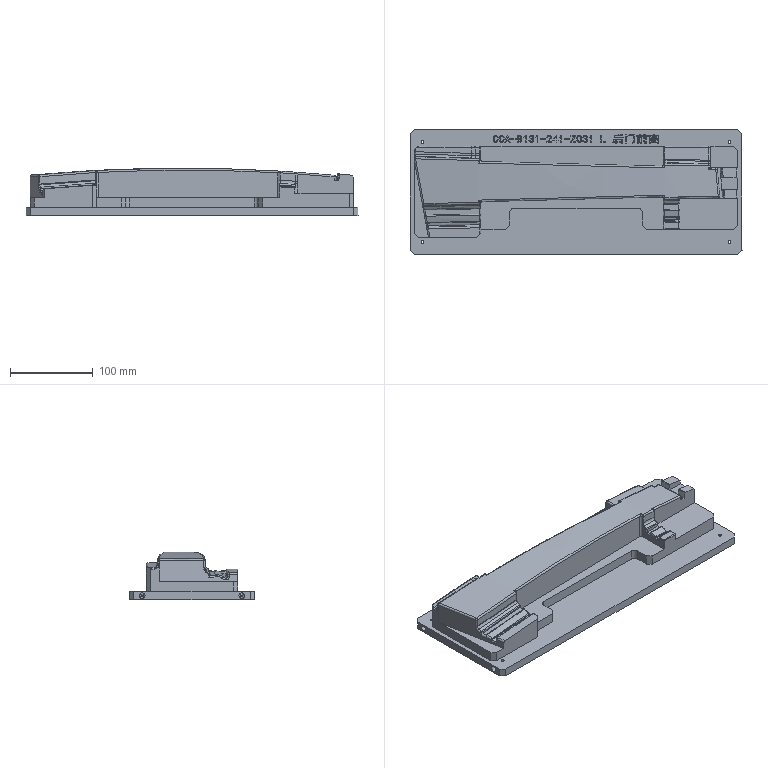NC program | NX | posted with a generic post | part box 400 x 150 x 57.494 mm
Lines 7336 to 8369 of 16235:
(B2 , TOOL : D6)
N14670 M6
N14672 G54
N14674 G17 G0 G90 X-117.012 Y45.277 S3500 M3
N14676 G43 Z69.953 H0
N14678 Z54.94
N14680 G94 G1 Z54.64 F2000.
N14682 X-115.309 Y43.211
N14684 X-113.402 Y40.898 Z54.536
N14686 G2 X-112.655 Y39.453 R3.866
N14688 X-109.882 Y39.507 R578.074
N14690 G1 X-106.884 Y39.558 Z54.64
N14692 X-106.919 Y42.55
N14694 Z54.94
N14696 G0 Z62.753
N14698 X-116.766 Y45.803
N14700 Z54.445
N14702 G1 Z54.145
N14704 X-114.899 Y43.597
N14706 X-112.963 Y41.308 Z54.041
N14708 G2 X-112.167 Y39.876 R4.223
N14710 X-109.559 Y39.87 R984.3
N14712 G1 X-106.561 Y39.859 Z54.145
N14714 X-106.541 Y42.854
N14716 Z54.445
N14718 G0 Z54.836
N14720 X-116.488 Y46.083
N14722 Z53.951
N14724 G1 Z53.651
N14726 X-114.599 Y43.8
N14728 X-112.687 Y41.491 Z53.546
N14730 G2 X-111.905 Y40.082 R4.383
N14732 X-109.285 Y40.044 R1249.651
N14734 G1 X-106.287 Y39.998 Z53.651
N14736 X-106.234 Y42.994
N14738 Z53.951
N14740 G0 Z54.341
N14742 X-116.36 Y46.216
N14744 Z53.456
N14746 G1 Z53.156
N14748 X-114.458 Y43.892
N14750 X-112.56 Y41.572 Z53.051
N14752 G2 X-111.787 Y40.176 R4.458
N14754 G1 X-109.211 Y40.108
N14756 X-106.213 Y40.03 Z53.156
N14758 X-106.135 Y43.029
N14760 Z53.456
N14762 G0 Z53.846
N14764 X-116.319 Y46.25
N14766 Z52.961
N14768 G1 Z52.661
N14770 X-114.409 Y43.907
N14772 X-112.514 Y41.583 Z52.556
N14774 G2 X-111.738 Y40.18 R4.504
N14776 G1 X-109.189 Y40.113
N14778 X-106.192 Y40.035 Z52.661
N14780 X-106.114 Y43.034
N14782 Z52.961
N14784 G0 Z53.351
N14786 X-116.324 Y46.252
N14788 Z52.466
N14790 G1 Z52.166
N14792 X-114.411 Y43.908
N14794 X-112.515 Y41.585 Z52.062
N14796 G2 X-111.738 Y40.18 R4.503
N14798 G1 X-109.188 Y40.113
N14800 X-106.191 Y40.035 Z52.166
N14802 X-106.113 Y43.034
N14804 Z52.466
N14806 G0 Z52.856
N14808 X-116.328 Y46.252
N14810 Z51.971
N14812 G1 Z51.671
N14814 X-114.413 Y43.909
N14816 X-112.517 Y41.587 Z51.567
N14818 G2 X-111.741 Y40.187 R4.502
N14820 G1 X-111.529 Y40.175
N14822 X-109.188 Y40.113
N14824 X-106.191 Y40.035 Z51.671
N14826 X-106.112 Y43.034
N14828 Z51.971
N14830 G0 Z52.362
N14832 X-116.331 Y46.252
N14834 Z51.477
N14836 G1 Z51.177
N14838 X-114.416 Y43.91
N14840 X-112.518 Y41.589 Z51.072
N14842 G2 X-111.741 Y40.187 R4.501
N14844 G1 X-111.529 Y40.175
N14846 X-109.187 Y40.113
N14848 X-106.19 Y40.035 Z51.177
N14850 X-106.111 Y43.034
N14852 Z51.477
N14854 G0 Z51.867
N14856 X-116.334 Y46.253
N14858 Z50.982
N14860 G1 Z50.682
N14862 X-114.418 Y43.911
N14864 X-112.519 Y41.591 Z50.577
N14866 G2 X-111.741 Y40.187 R4.5
N14868 G1 X-111.529 Y40.175
N14870 X-109.186 Y40.113
N14872 X-106.189 Y40.035 Z50.682
N14874 X-106.11 Y43.034
N14876 Z50.982
N14878 G0 Z51.372
N14880 X-116.332 Y46.251
N14882 Z50.487
N14884 G1 Z50.187
N14886 X-114.418 Y43.911
N14888 X-112.519 Y41.591 Z50.082
N14890 G2 X-111.741 Y40.187 R4.498
N14892 G1 X-111.681 Y40.177
N14894 X-111.529 Y40.172
N14896 Y40.175
N14898 X-109.186 Y40.113
N14900 X-106.189 Y40.035 Z50.187
N14902 X-106.11 Y43.034
N14904 Z50.487
N14906 G0 Z50.877
N14908 X-116.333 Y46.253
N14910 Z49.992
N14912 G1 Z49.692
N14914 X-114.418 Y43.912
N14916 X-112.519 Y41.591 Z49.587
N14918 G2 X-111.74 Y40.187 R4.497
N14920 G1 X-111.681 Y40.177
N14922 X-111.529 Y40.175
N14924 X-109.186 Y40.113
N14926 X-106.188 Y40.035 Z49.692
N14928 X-106.11 Y43.034
N14930 Z49.992
N14932 G0 Z50.382
N14934 X-116.332 Y46.253
N14936 Z49.497
N14938 G1 Z49.197
N14940 X-114.417 Y43.912
N14942 X-112.519 Y41.592 Z49.093
N14944 G2 X-111.74 Y40.187 R4.496
N14946 G1 X-111.681 Y40.177
N14948 X-111.529 Y40.175
N14950 X-109.185 Y40.113
N14952 X-106.188 Y40.035 Z49.197
N14954 X-106.11 Y43.034
N14956 Z49.497
N14958 G0 Z49.887
N14960 X-116.333 Y46.253
N14962 Z49.003
N14964 G1 Z48.703
N14966 X-114.417 Y43.912
N14968 X-112.518 Y41.591 Z48.598
N14970 G2 X-111.747 Y40.208 R4.498
N14972 G1 X-111.737 Y40.165
N14974 X-111.696 Y40.179
N14976 X-109.185 Y40.113
N14978 X-106.188 Y40.035 Z48.703
N14980 X-106.109 Y43.034
N14982 Z49.003
N14984 G0 Z49.393
N14986 X-116.331 Y46.251
N14988 Z48.508
N14990 G1 Z48.208
N14992 X-114.417 Y43.912
N14994 X-112.518 Y41.592 Z48.103
N14996 G2 X-111.746 Y40.208 R4.497
N14998 G1 X-111.737 Y40.164
N15000 X-111.695 Y40.179
N15002 X-109.185 Y40.113
N15004 X-106.187 Y40.035 Z48.208
N15006 X-106.109 Y43.034
N15008 Z48.508
N15010 G0 Z48.898
N15012 X-116.324 Y46.251
N15014 Z48.013
N15016 G1 Z47.713
N15018 X-114.413 Y43.912
N15020 X-112.516 Y41.59 Z47.608
N15022 G2 X-111.746 Y40.208 R4.494
N15024 G1 X-111.737 Y40.164
N15026 X-111.695 Y40.179
N15028 X-109.184 Y40.113
N15030 X-106.187 Y40.035 Z47.713
N15032 X-106.109 Y43.034
N15034 Z48.013
N15036 G0 Z48.403
N15038 X-116.302 Y46.271
N15040 Z47.518
N15042 G1 Z47.218
N15044 X-114.399 Y43.923
N15046 X-112.511 Y41.595 Z47.113
N15048 G2 X-111.738 Y40.188 R4.505
N15050 G1 X-111.678 Y40.179
N15052 X-109.174 Y40.113
N15054 X-106.177 Y40.035 Z47.218
N15056 X-106.098 Y43.034
N15058 Z47.518
N15060 G0 Z47.908
N15062 X-116.122 Y46.434
N15064 Z47.023
N15066 G1 Z46.723
N15068 X-114.299 Y44.065
N15070 X-112.47 Y41.69 Z46.619
N15072 G2 X-112.002 Y40.938 R4.471
N15074 G1 X-111.717 Y40.316
N15076 X-111.748 Y40.233
N15078 X-111.678 Y40.179
N15080 X-109.013 Y40.109
N15082 X-106.015 Y40.03 Z46.723
N15084 X-105.937 Y43.029
N15086 Z47.023
N15088 G0 Z47.413
N15090 X-115.811 Y46.744
N15092 Z46.528
N15094 G1 Z46.228
N15096 X-114.099 Y44.296
N15098 X-112.38 Y41.84 Z46.124
N15100 G2 X-111.86 Y40.855 R4.471
N15102 G1 X-111.656 Y40.316
N15104 X-111.642 Y40.178
N15106 X-108.697 Y40.101
N15108 X-105.699 Y40.022 Z46.228
N15110 X-105.621 Y43.021
N15112 Z46.528
N15114 G0 Z46.919
N15116 X-115.417 Y47.282
N15118 Z46.034
N15120 G1 Z45.734
N15122 X-113.898 Y44.752
N15124 X-112.354 Y42.182 Z45.629
N15126 X-112.236 Y41.987
N15128 G2 X-111.576 Y40.176 R5.063
N15130 G1 X-108.345 Y40.092
N15132 X-105.348 Y40.013 Z45.734
N15134 X-105.27 Y43.012
N15136 Z46.034
N15138 G0 Z46.424
N15140 X-115.223 Y48.184
N15142 Z45.539
N15144 G1 Z45.239
N15146 X-113.671 Y45.306
N15148 X-112.249 Y42.667 Z45.134
N15150 G2 X-111.524 Y40.224 R6.224
N15152 G1 X-111.54 Y40.181
N15154 X-111.503 Y40.149
N15156 X-111.462 Y40.17
N15158 X-107.74 Y40.073
N15160 X-104.743 Y39.994 Z45.239
N15162 X-104.664 Y42.993
N15164 Z45.539
N15166 G0 Z45.929
N15168 X-109.191 Y48.973
N15170 Z45.044
N15172 G1 Z44.744
N15174 X-112.19 Y48.917
N15176 X-112.134 Y45.919 Z44.639
N15178 X-112.093 Y43.733
N15180 X-112.056 Y43.424
N15182 G2 X-111.5 Y40.29 R12.132
N15184 G1 Y40.175
N15186 X-106.26 Y40.038
N15188 X-103.262 Y39.959 Z44.744
N15190 X-103.184 Y42.958
N15192 Z45.044
N15194 G0 Z45.434
N15196 X-108.67 Y49.116
N15198 Z44.549
N15200 G1 Z44.249
N15202 X-111.67 Y49.102
N15204 X-111.656 Y46.104 Z44.144
N15206 X-111.644 Y43.424
N15208 X-111.515 Y41.559
N15210 X-111.5 Y41.107
N15212 Y40.175
N15214 X-105.75 Y40.024
N15216 X-102.753 Y39.946 Z44.249
N15218 X-102.674 Y42.945
N15220 Z44.549
N15222 G0 Z44.939
N15224 X-108.509 Y49.092
N15226 Z44.054
N15228 G1 Z43.754
N15230 X-111.509 Y49.088
N15232 X-111.506 Y46.09 Z43.65
N15234 X-111.502 Y42.802
N15236 X-111.5 Y42.704
N15238 Y40.175
N15240 X-105.601 Y40.02
N15242 X-102.604 Y39.942 Z43.754
N15244 X-102.525 Y42.941
N15246 Z44.054
N15248 G0 Z44.444
N15250 X-108.5 Y49.074
N15252 Z43.56
N15254 G1 Z43.26
N15256 X-111.5
N15258 Y46.076 Z43.155
N15260 Y40.175
N15262 X-105.601 Y40.02
N15264 X-102.604 Y39.942 Z43.26
N15266 X-102.525 Y42.941
N15268 Z43.56
N15270 G0 Z43.95
N15272 X-108.5 Y49.074
N15274 Z43.065
N15276 G1 Z42.765
N15278 X-111.5
N15280 Y46.076 Z42.66
N15282 Y40.175
N15284 X-105.601 Y40.02
N15286 X-102.603 Y39.942 Z42.765
N15288 X-102.525 Y42.941
N15290 Z43.065
N15292 G0 Z43.455
N15294 X-108.5 Y49.074
N15296 Z42.57
N15298 G1 Z42.27
N15300 X-111.5
N15302 Y46.076 Z42.165
N15304 Y40.175
N15306 X-105.6 Y40.02
N15308 X-102.603 Y39.942 Z42.27
N15310 X-102.525 Y42.941
N15312 Z42.57
N15314 G0 Z42.96
N15316 X-108.5 Y49.074
N15318 Z42.075
N15320 G1 Z41.775
N15322 X-111.5
N15324 Y46.076 Z41.67
N15326 Y40.175
N15328 X-105.6 Y40.02
N15330 X-102.603 Y39.942 Z41.775
N15332 X-102.524 Y42.941
N15334 Z42.075
N15336 G0 Z42.465
N15338 X-108.5 Y49.074
N15340 Z41.58
N15342 G1 Z41.28
N15344 X-111.5
N15346 Y46.076 Z41.176
N15348 Y40.175
N15350 X-105.6 Y40.02
N15352 X-102.603 Y39.942 Z41.28
N15354 X-102.524 Y42.941
N15356 Z41.58
N15358 G0 Z41.97
N15360 X-108.5 Y49.074
N15362 Z41.085
N15364 G1 Z40.785
N15366 X-111.5
N15368 Y46.076 Z40.681
N15370 Y40.175
N15372 X-105.6 Y40.02
N15374 X-102.603 Y39.942 Z40.785
N15376 X-102.524 Y42.941
N15378 Z41.085
N15380 G0 Z41.476
N15382 X-108.5 Y49.074
N15384 Z40.591
N15386 G1 Z40.291
N15388 X-111.5
N15390 Y46.076 Z40.186
N15392 Y40.175
N15394 X-105.6 Y40.02
N15396 X-102.602 Y39.942 Z40.291
N15398 X-102.524 Y42.941
N15400 Z40.591
N15402 G0 Z40.981
N15404 X-108.5 Y49.074
N15406 Z40.096
N15408 G1 Z39.796
N15410 X-111.5
N15412 Y46.076 Z39.691
N15414 Y40.175
N15416 X-105.599 Y40.02
N15418 X-102.602 Y39.942 Z39.796
N15420 X-102.524 Y42.941
N15422 Z40.096
N15424 G0 Z40.486
N15426 X-108.5 Y49.074
N15428 Z39.601
N15430 G1 Z39.301
N15432 X-111.5
N15434 Y46.076 Z39.196
N15436 Y40.175
N15438 X-105.599 Y40.02
N15440 X-102.602 Y39.942 Z39.301
N15442 X-102.524 Y42.941
N15444 Z39.601
N15446 G0 Z39.991
N15448 X-108.5 Y49.074
N15450 Z39.106
N15452 G1 Z38.806
N15454 X-111.5
N15456 Y46.076 Z38.702
N15458 Y40.175
N15460 X-105.599 Y40.02
N15462 X-102.602 Y39.942 Z38.806
N15464 X-102.523 Y42.941
N15466 Z39.106
N15468 G0 Z39.496
N15470 X-108.5 Y49.074
N15472 Z38.611
N15474 G1 Z38.311
N15476 X-111.5
N15478 Y46.076 Z38.207
N15480 Y40.175
N15482 X-105.599 Y40.02
N15484 X-102.602 Y39.942 Z38.311
N15486 X-102.523 Y42.941
N15488 Z38.611
N15490 G0 Z39.002
N15492 X-108.5 Y49.074
N15494 Z38.117
N15496 G1 Z37.817
N15498 X-111.5
N15500 Y46.076 Z37.712
N15502 Y40.175
N15504 X-105.599 Y40.02
N15506 X-102.601 Y39.942 Z37.817
N15508 X-102.523 Y42.941
N15510 Z38.117
N15512 G0 Z38.507
N15514 X-108.5 Y49.074
N15516 Z37.622
N15518 G1 Z37.322
N15520 X-111.5
N15522 Y46.076 Z37.217
N15524 Y40.175
N15526 X-105.598 Y40.02
N15528 X-102.601 Y39.942 Z37.322
N15530 X-102.523 Y42.941
N15532 Z37.622
N15534 G0 Z38.012
N15536 X-108.5 Y49.074
N15538 Z37.127
N15540 G1 Z36.827
N15542 X-111.5
N15544 Y46.076 Z36.722
N15546 Y40.175
N15548 X-105.598 Y40.02
N15550 X-102.601 Y39.942 Z36.827
N15552 X-102.523 Y42.941
N15554 Z37.127
N15556 G0 Z37.517
N15558 X-108.5 Y49.074
N15560 Z36.632
N15562 G1 Z36.332
N15564 X-111.5
N15566 Y46.076 Z36.227
N15568 Y40.175
N15570 X-105.598 Y40.02
N15572 X-102.601 Y39.942 Z36.332
N15574 X-102.522 Y42.941
N15576 Z36.632
N15578 G0 Z37.022
N15580 X-108.5 Y49.074
N15582 Z36.137
N15584 G1 Z35.837
N15586 X-111.5
N15588 Y46.076 Z35.733
N15590 Y40.175
N15592 X-105.598 Y40.02
N15594 X-102.601 Y39.942 Z35.837
N15596 X-102.522 Y42.941
N15598 Z36.137
N15600 G0 Z36.527
N15602 X-108.5 Y49.074
N15604 Z35.643
N15606 G1 Z35.343
N15608 X-111.5
N15610 Y46.076 Z35.238
N15612 Y40.175
N15614 X-105.598 Y40.02
N15616 X-102.601 Y39.942 Z35.343
N15618 X-102.522 Y42.941
N15620 Z35.643
N15622 G0 Z36.033
N15624 X-108.5 Y49.074
N15626 Z35.204
N15628 G1 Z34.904
N15630 X-111.5
N15632 Y46.076 Z34.799
N15634 Y40.175
N15636 X-105.597 Y40.02
N15638 X-102.6 Y39.942 Z34.904
N15640 X-102.522 Y42.941
N15642 Z35.204
N15644 G0 Z35.538
N15646 X-108.5 Y49.074
N15648 Z34.765
N15650 G1 Z34.465
N15652 X-111.5
N15654 Y46.076 Z34.361
N15656 Y40.175
N15658 X-105.597 Y40.02
N15660 X-102.6 Y39.942 Z34.465
N15662 X-102.522 Y42.941
N15664 Z34.765
N15666 G0 Z35.099
N15668 X-108.5 Y49.074
N15670 Z34.327
N15672 G1 Z34.027
N15674 X-111.5
N15676 Y46.076 Z33.922
N15678 Y40.175
N15680 X-105.597 Y40.02
N15682 X-102.6 Y39.942 Z34.027
N15684 X-102.521 Y42.941
N15686 Z34.327
N15688 G0 Z34.661
N15690 X-108.5 Y49.074
N15692 Z33.888
N15694 G1 Z33.588
N15696 X-111.5
N15698 Y46.076 Z33.483
N15700 Y40.175
N15702 X-105.597 Y40.02
N15704 X-102.6 Y39.942 Z33.588
N15706 X-102.521 Y42.941
N15708 Z33.888
N15710 G0 Z34.222
N15712 X-108.5 Y49.074
N15714 Z33.449
N15716 G1 Z33.149
N15718 X-111.5
N15720 Y46.076 Z33.045
N15722 Y40.175
N15724 X-105.597 Y40.02
N15726 X-102.6 Y39.942 Z33.149
N15728 X-102.521 Y42.941
N15730 Z33.449
N15732 G0 Z69.954
N15734 X-127.447 Y48.251 Z69.951
N15736 Z44.939
N15738 G1 Z44.639
N15740 X-126.863 Y45.297
N15742 G3 X-122.642 Y45.838 R124.669
N15744 G1 X-122.517 Y46.532
N15746 X-121.921 Y50.078
N15748 X-121.423 Y53.035 Z44.744
N15750 X-120.424 Y58.973
N15752 Z45.044
N15754 G0 Z45.434
N15756 X-137.602 Y48.249
N15758 Z44.497
N15760 G1 Z44.197
N15762 X-137.362 Y45.254
N15764 X-135.868 Y45.383 Z44.144
N15766 X-135.858 Y45.384
N15768 X-131.492 Y45.945
N15770 X-131.305 Y45.977
N15772 X-130.637 Y50.421
N15774 X-130.19 Y53.385 Z44.249
N15776 X-129.339 Y59.043
N15778 Z44.549
N15780 G0 Z44.939
N15782 X-144.276 Y48.585
N15784 Z43.95
N15786 G1 Z43.65
N15788 X-143.686 Y45.631
N15790 G3 X-139.369 Y46.174 R142.581
N15792 X-138.693 Y50.687 R78.701
N15794 G1 X-141.646 Y51.267
N15796 Z43.95
N15798 G0 Z44.444
N15800 X-151.988 Y48.676
N15802 Z43.455
N15804 G1 Z43.155
N15806 X-151.373 Y45.732
N15808 X-147.711 Y46.228
N15810 X-146.943 Y46.363
N15812 G3 X-146.323 Y50.908 R269.108
N15814 G1 X-149.276 Y51.471
N15816 Z43.455
N15818 G0 Z43.95
N15820 X-161.639 Y48.651
N15822 Z43.065
N15824 G1 Z42.765
N15826 X-161.354 Y45.665
N15828 X-158.37 Y45.949 Z42.66
N15830 X-155.821 Y46.191
N15832 X-154.05 Y46.519
N15834 G3 X-153.422 Y51.422 R90.292
N15836 G1 X-156.393 Y51.865
N15838 Z42.96
N15840 G0 Z43.455
N15842 X-166.049 Y48.967
N15844 Z42.465
N15846 G1 Z42.165
N15848 X-165.456 Y46.017
N15850 G3 X-160.829 Y46.733 R76.993
N15852 G1 X-160.347 Y51.362
N15854 X-160.036 Y54.344 Z42.27
N15856 X-159.556 Y58.951
N15858 Z42.57
N15860 G0 Z42.96
N15862 X-172.625 Y49.09
N15864 Z41.97
N15866 G1 Z41.67
N15868 X-172.081 Y46.132
N15870 G3 X-167.335 Y46.83 R68.397
N15872 G1 X-166.79 Y50.882
N15874 G2 X-166.775 Y51.806 R25.204
N15876 G1 X-166.669 Y54.802 Z41.775
N15878 X-166.532 Y58.685
N15880 Z42.075
N15882 G0 Z42.465
N15884 X-178.894 Y49.228
N15886 Z41.476
N15888 G1 Z41.176
N15890 X-178.36 Y46.267
N15892 X-178.278 Y46.276
N15894 X-173.539 Y46.995
N15896 X-173.113 Y51.631
N15898 X-172.839 Y54.617 Z41.28
N15900 X-172.446 Y58.903
N15902 Z41.58
N15904 G0 Z41.97
N15906 X-184.831 Y49.354
N15908 Z40.981
N15910 G1 Z40.681
N15912 X-184.251 Y46.403
N15914 G3 X-179.503 Y47.158 R72.333
N15916 X-179.025 Y52.052 R124.303
N15918 G1 X-182.004 Y52.441
N15920 Z40.981
N15922 G0 Z41.476
N15924 X-190.782 Y49.444
N15926 Z40.486
N15928 G1 Z40.186
N15930 X-190.264 Y46.484
N15932 G3 X-185.247 Y47.262 R62.292
N15934 G1 X-184.815 Y52.125
N15936 X-184.818 Y52.351
N15938 X-184.857 Y55.349 Z40.291
N15940 X-184.899 Y58.529
N15942 Z40.591
N15944 G0 Z40.981
N15946 X-200.687 Y44.368
N15948 Z40.096
N15950 G1 Z39.796
N15952 X-196.942 Y45.757
N15954 X-194.131 Y46.8 Z39.691
N15956 X-193.874 Y46.895
N15958 X-190.81 Y47.411
N15960 X-190.524 Y51.625
N15962 X-190.32 Y54.616 Z39.796
N15964 X-190.036 Y58.809
N15966 Z40.096
N15968 G0 Z40.486
N15970 X-201.5 Y38.971
N15972 Z39.601
N15974 G1 Z39.301
N15976 X-198.33 Y43.672
N15978 X-196.653 Y46.157 Z39.196
N15980 G2 X-196.283 Y46.67 R10.016
N15982 G1 X-196.232 Y47.415
N15984 X-196.029 Y50.406 Z39.301
N15986 X-195.473 Y58.598
N15988 Z39.601
N15990 G0 Z69.947
N15992 X-128.079 Y-31.338 Z69.984
N15994 Z35.643
N15996 G1 Z35.343
N15998 X-125.324 Y-31.22
N16000 X-125.827 Y-28.264 Z35.238
N16002 G2 X-124.869 Y-25.396 R3.208
N16004 G1 X-124.391 Y-24.944
N16006 X-123.682 Y-24.595
N16008 G2 X-121.244 Y-23.918 R6.881
N16010 X-131.585 Y-24.043 R537.118
N16012 G1 X-134.583 Y-24.05 Z35.343
N16014 X-134.593 Y-27.042
N16016 Z35.643
N16018 G0 Z36.033
N16020 X-135.303 Y-30.845
N16022 Z35.152
N16024 G1 Z34.852
N16026 X-132.425 Y-30.218
N16028 X-132.836 Y-28.776 Z34.799
N16030 G2 X-130.868 Y-24.689 R3.412
N16032 G1 X-128.548 Y-24.081
N16034 X-128.507 Y-24.074
N16036 G2 X-138.677 Y-24.192 R431.764
N16038 G1 X-141.675 Y-24.191 Z34.904
N16040 X-141.696 Y-27.181
N16042 Z35.204
N16044 G0 Z35.538
N16046 X-141.857 Y-31.68
N16048 Z34.765
N16050 G1 Z34.465
N16052 X-139.1 Y-31.55
N16054 X-139.613 Y-28.596 Z34.361
N16056 G2 X-138.354 Y-25.407 R3.29
N16058 X-137.357 Y-24.783 R2.013
N16060 G1 X-135.262 Y-24.219
N16062 G2 X-145.3 Y-24.326 R468.182
N16064 G1 X-148.298 Z34.465
N16066 X-148.317 Y-27.316
N16068 Z34.765
N16070 G0 Z35.099
N16072 X-148.194 Y-31.904
N16074 Z34.327
N16076 G1 Z34.027
N16078 X-145.216 Y-31.826
N16080 X-145.883 Y-28.903 Z33.922
N16082 G2 X-143.344 Y-24.807 R3.428
N16084 G1 X-141.76 Y-24.368
N16086 X-141.711 Y-24.36
N16088 G2 X-151.669 Y-24.447 R378.56
N16090 G1 X-154.667 Y-24.434 Z34.027
N16092 X-154.704 Y-27.421
N16094 Z34.327
N16096 G0 Z34.661
N16098 X-154.284 Y-31.959
N16100 Z33.888
N16102 G1 Z33.588
N16104 X-151.448 Y-31.841
N16106 X-152.019 Y-28.897 Z33.483
N16108 G2 X-150.725 Y-25.565 R3.355
N16110 G1 X-150.206 Y-25.277
N16112 G2 X-147.819 Y-24.489 R6.344
N16114 X-157.708 Y-24.57 R331.462
N16116 G1 X-160.706 Y-24.55 Z33.588
N16118 X-160.753 Y-27.537
N16120 Z33.888
N16122 G0 Z34.222
N16124 X-160.072 Y-32.067
N16126 Z33.449
N16128 G1 Z33.149
N16130 X-157.232 Y-31.96
N16132 X-157.796 Y-29.015 Z33.045
N16134 G2 X-156.094 Y-25.449 R3.332
N16136 X-153.663 Y-24.615 R8.054
N16138 X-163.511 Y-24.68 R352.859
N16140 G1 X-166.509 Y-24.658 Z33.149
N16142 X-166.556 Y-27.645
N16144 Z33.449
N16146 G0 Z33.783
N16148 X-165.736 Y-31.443
N16150 Z32.958
N16152 G1 Z32.658
N16154 X-162.877 Y-30.827
N16156 X-163.26 Y-29.378 Z32.606
N16158 G2 X-162.883 Y-26.723 R3.451
N16160 X-161.435 Y-25.396 R3.877
N16162 G1 X-159.301 Y-24.734
N16164 G2 X-169.096 Y-24.796 R360.815
N16166 G1 X-172.094 Y-24.774 Z32.711
N16168 X-172.148 Y-27.761
N16170 Z33.011
N16172 G0 Z33.345
N16174 X-171.168 Y-31.484
N16176 Z32.52
N16178 G1 Z32.22
N16180 X-168.357 Y-30.855
N16182 X-168.7 Y-29.396 Z32.167
N16184 G2 X-166.412 Y-25.37 R3.405
N16186 G1 X-164.759 Y-24.847
N16188 G2 X-174.448 Y-24.895 R302.322
N16190 G1 X-177.446 Y-24.861 Z32.272
N16192 X-177.509 Y-27.846
N16194 Z32.572
N16196 G0 Z32.906
N16198 X-176.145 Y-32.437
N16200 Z32.133
N16202 G1 Z31.833
N16204 X-173.262 Y-32.348
N16206 X-173.844 Y-29.407 Z31.729
N16208 G2 X-172.475 Y-25.976 R3.395
N16210 G1 X-172.04 Y-25.669
N16212 X-171.896 Y-25.565
N16214 X-170.169 Y-25.015
N16216 X-169.893 Y-24.956
N16218 G2 X-179.523 Y-24.997 R330.395
N16220 G1 X-182.521 Y-24.965 Z31.833
N16222 X-188.54 Y-24.903
N16224 Z32.133
N16226 G0 Z32.467
N16228 X-181.243 Y-32.975
N16230 Z31.638
N16232 G1 Z31.338
N16234 X-179.343 Y-32.195
N16236 X-179.658 Y-29.213 Z31.234
N16238 G2 X-178.068 Y-25.985 R3.372
N16240 G1 X-177.384 Y-25.565
N16242 X-175.783 Y-25.1
N16244 X-175.678 Y-25.079
N16246 X-182.138 Y-25.145
N16248 G2 X-183.407 Y-24.992 R5.438
N16250 G1 X-186.321 Y-24.288 Z31.338
N16252 X-189.679 Y-23.477
N16254 Z31.638
N16256 G0 Z32.029
N16258 X-185.461 Y-33.67
N16260 Z31.143
N16262 G1 Z30.843
N16264 X-184.894 Y-31.102
N16266 X-184.248 Y-28.175 Z30.739
N16268 G2 X-182.489 Y-25.74 R3.779
N16270 G1 X-182.044 Y-25.476
N16272 X-181.165 Y-25.19
N16274 X-182.023 Y-25.205
N16276 G2 X-185.731 Y-23.864 R5.5
N16278 G1 X-187.997 Y-21.901 Z30.843
N16280 X-190.817 Y-19.459
N16282 Z31.143
N16284 G0 Z31.534
N16286 X-186.473 Y-33.975
N16288 Z30.648
N16290 G1 Z30.348
N16292 X-185.693 Y-30.955
N16294 X-184.943 Y-28.052 Z30.244
N16296 G2 X-182.701 Y-25.209 R4.489
N16298 G1 X-183.811 Y-24.944
N16300 X-184.235 Y-24.802
N16302 G2 X-186.06 Y-23.554 R5.565
N16304 G1 X-188.15 Y-21.404 Z30.348
N16306 X-190.997 Y-18.475
N16308 Z30.648
N16310 G0 Z31.039
N16312 X-187.105 Y-34.073
N16314 Z30.153
N16316 G1 Z29.853
N16318 X-186.116 Y-30.836
N16320 X-185.24 Y-27.969 Z29.749
N16322 G2 X-182.975 Y-25.151 R4.867
N16324 X-186.199 Y-23.404 R5.533
N16326 G1 X-188.213 Y-21.183 Z29.853
N16328 X-191.08 Y-18.021
N16330 Z30.153
N16332 G0 Z30.544
N16334 X-188.511 Y-26.55
N16336 Z29.606
N16338 G1 Z29.306
N16340 X-185.551 Y-26.061
N16342 X-185.796 Y-24.582 Z29.254
N16344 X-185.948 Y-23.665
N16346 G2 X-186.377 Y-23.201 R5.487
N16348 G1 X-188.283 Y-20.888 Z29.358
N16350 X-191.204 Y-17.344
N16352 Z29.658
N16354 G0 Z30.049
N16356 X-188.993 Y-26.85
N16358 Z29.163
N16360 G1 Z28.863
N16362 X-186.036 Y-26.341
N16364 X-186.545 Y-23.386 Z28.759
N16366 X-186.633 Y-22.878
N16368 G2 X-186.78 Y-22.653 R5.68
N16370 G1 X-188.364 Y-20.107 Z28.863
N16372 X-191.672 Y-14.786
N16374 Z29.163
N16376 G0 Z69.977
N16378 X-187.458 Y-34.359 Z69.985
N16380 Z29.658
N16382 G1 Z29.358
N16384 X-186.347 Y-30.931
N16386 X-185.423 Y-28.078 Z29.254
N16388 G2 X-185.272 Y-27.676 R4.86
N16390 G1 X-185.325 Y-27.43
N16392 X-185.387 Y-27.057
N16394 X-185.876 Y-24.099 Z29.358
N16396 X-188.758 Y-25.183
N16398 Z29.658
N16400 G0 Z30.049
N16402 X-187.058 Y-36.308
N16404 Z29.163
N16406 G1 Z28.863
N16408 X-186.214 Y-31.802
N16410 X-185.662 Y-28.856 Z28.759
N16412 X-185.63 Y-28.699
N16414 X-185.682 Y-28.394
N16416 X-186.192 Y-25.44 Z28.863
N16418 X-189.148 Y-25.949
N16420 Z29.163
N16422 G0 Z69.982
N16424 X-103.976 Y-51.495 Z69.992
N16426 Z22.233
N16428 G1 Z21.933
N16430 Y-48.495
N16432 X-106.974 Z21.829
N16434 X-111.5
N16436 Y-49.995
N16438 G2 X-111.775 Y-51.356 R3.5
N16440 G1 X-112.941 Y-54.118 Z21.933
N16442 X-115.14 Y-59.328
N16444 Z22.233
N16446 G0 Z22.624
N16448 X-103.976 Y-51.495
N16450 Z21.738
N16452 G1 Z21.438
N16454 Y-48.495
N16456 X-106.974 Z21.334
N16458 X-111.5
N16460 Y-49.995
N16462 G2 X-111.775 Y-51.356 R3.5
N16464 G1 X-112.941 Y-54.118 Z21.438
N16466 X-115.139 Y-59.327
N16468 Z21.738
N16470 G0 Z22.129
N16472 X-103.976 Y-51.496
N16474 Z21.243
N16476 G1 Z20.943
N16478 Y-48.496
N16480 X-106.975 Z20.839
N16482 X-111.5
N16484 Y-49.996
N16486 G2 X-111.775 Y-51.356 R3.5
N16488 G1 X-112.941 Y-54.119 Z20.943
N16490 X-115.139 Y-59.327
N16492 Z21.243
N16494 G0 Z21.634
N16496 X-103.976 Y-51.496
N16498 Z20.748
N16500 G1 Z20.448
N16502 Y-48.496
N16504 X-106.975 Z20.344
N16506 X-111.5
N16508 Y-49.996
N16510 G2 X-111.775 Y-51.356 R3.5
N16512 G1 X-112.941 Y-54.119 Z20.448
N16514 X-115.138 Y-59.326
N16516 Z20.748
N16518 G0 Z21.139
N16520 X-103.976 Y-51.496
N16522 Z20.253
N16524 G1 Z19.953
N16526 Y-48.496
N16528 X-106.975 Z19.849
N16530 X-111.5
N16532 Y-49.996
N16534 G2 X-111.775 Y-51.356 R3.5
N16536 G1 X-112.941 Y-54.119 Z19.953
N16538 X-115.137 Y-59.326
N16540 Z20.253
N16542 G0 Z20.644
N16544 X-103.977 Y-51.496
N16546 Z19.758
N16548 G1 Z19.458
N16550 Y-48.496
N16552 X-106.975 Z19.354
N16554 X-111.5
N16556 Y-49.996
N16558 G2 X-111.775 Y-51.356 R3.5
N16560 G1 X-112.94 Y-54.119 Z19.458
N16562 X-115.136 Y-59.325
N16564 Z19.758
N16566 G0 Z20.149
N16568 X-103.977 Y-51.496
N16570 Z19.263
N16572 G1 Z18.963
N16574 Y-48.496
N16576 X-106.975 Z18.859
N16578 X-111.5
N16580 Y-49.996
N16582 G2 X-111.775 Y-51.357 R3.5
N16584 G1 X-112.94 Y-54.119 Z18.963
N16586 X-115.136 Y-59.324
N16588 Z19.263
N16590 G0 Z19.654
N16592 X-103.977 Y-51.497
N16594 Z18.768
N16596 G1 Z18.468
N16598 Y-48.497
N16600 X-106.975 Z18.364
N16602 X-111.5
N16604 Y-49.997
N16606 G2 X-111.775 Y-51.357 R3.5
N16608 G1 X-112.94 Y-54.119 Z18.468
N16610 X-115.135 Y-59.324
N16612 Z18.768
N16614 G0 Z19.159
N16616 X-103.977 Y-51.497
N16618 Z18.273
N16620 G1 Z17.973
N16622 Y-48.497
N16624 X-106.975 Z17.869
N16626 X-111.5
N16628 Y-49.997
N16630 G2 X-111.775 Y-51.357 R3.5
N16632 G1 X-112.94 Y-54.119 Z17.973
N16634 X-115.134 Y-59.323
N16636 Z18.273
N16638 G0 Z18.664
N16640 X-103.977 Y-51.497
N16642 Z17.778
N16644 G1 Z17.478
N16646 Y-48.497
N16648 X-106.975 Z17.374
N16650 X-111.5
N16652 Y-49.997
N16654 G2 X-111.775 Y-51.357 R3.5
N16656 G1 X-112.94 Y-54.119 Z17.478
N16658 X-115.133 Y-59.323
N16660 Z17.778
N16662 G0 Z18.169
N16664 X-103.977 Y-51.497
N16666 Z17.283
N16668 G1 Z16.983
N16670 Y-48.497
N16672 X-106.975 Z16.879
N16674 X-111.5
N16676 Y-49.997
N16678 G2 X-111.775 Y-51.357 R3.5
N16680 G1 X-112.939 Y-54.119 Z16.983
N16682 X-115.133 Y-59.322
N16684 Z17.283
N16686 G0 Z17.674
N16688 X-103.977 Y-51.497
N16690 Z16.788
N16692 G1 Z16.488
N16694 Y-48.497
N16696 X-106.975 Z16.384
N16698 X-111.5
N16700 Y-49.997
N16702 G2 X-111.775 Y-51.357 R3.5
N16704 G1 X-112.939 Y-54.12 Z16.488
N16706 X-115.132 Y-59.322
N16708 Z16.788
N16710 G0 Z17.179
N16712 X-103.977 Y-51.498
N16714 Z16.293
N16716 G1 Z15.993
N16718 Y-48.498
N16720 X-106.975 Z15.889
N16722 X-111.5
N16724 Y-49.998
N16726 G2 X-111.775 Y-51.357 R3.5
N16728 G1 X-112.939 Y-54.12 Z15.993
N16730 X-115.131 Y-59.321